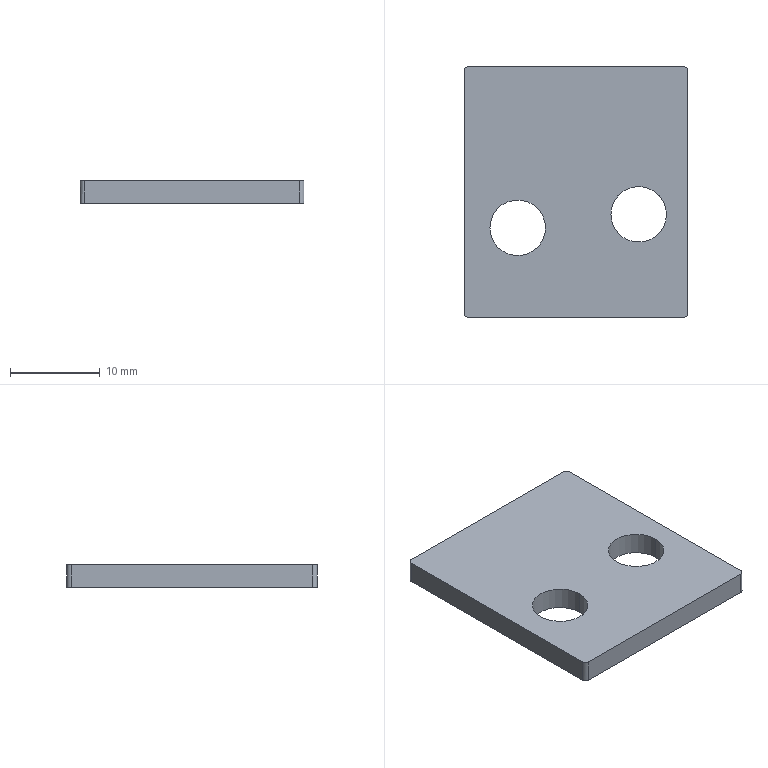Part | STEP file | PN_0024_Default<As Machined> | 1 solid | 14 faces | box 25 x 28 x 2.5 mm | volume 1599 mm3 | cylinder 8 | plane 6 | commonest cylinder face diameters 1 x4 6.2 x4
STEP:
#1=CARTESIAN_POINT('',(3.9,-2.5,2.5));
#2=VERTEX_POINT('',#1);
#3=CARTESIAN_POINT('',(10.1,-2.5,2.5));
#4=VERTEX_POINT('',#3);
#5=CARTESIAN_POINT('',(7.,-2.5,2.5));
#6=DIRECTION('',(0.,0.,-1.));
#7=AXIS2_PLACEMENT_3D('',#5,#6,$);
#8=CIRCLE('',#7,3.1);
#9=EDGE_CURVE('',#2,#4,#8,.F.);
#10=ORIENTED_EDGE('',*,*,#9,.T.);
#11=CARTESIAN_POINT('',(10.1,-2.5,0.));
#12=VERTEX_POINT('',#11);
#13=CARTESIAN_POINT('',(10.1,-2.5,2.5));
#14=DIRECTION('',(0.,0.,-1.));
#15=VECTOR('',#14,1.);
#16=LINE('',#13,#15);
#17=EDGE_CURVE('',#4,#12,#16,.T.);
#18=ORIENTED_EDGE('',*,*,#17,.T.);
#19=CARTESIAN_POINT('',(3.9,-2.5,0.));
#20=VERTEX_POINT('',#19);
#21=CARTESIAN_POINT('',(7.,-2.5,0.));
#22=DIRECTION('',(0.,0.,-1.));
#23=AXIS2_PLACEMENT_3D('',#21,#22,$);
#24=CIRCLE('',#23,3.1);
#25=EDGE_CURVE('',#20,#12,#24,.F.);
#26=ORIENTED_EDGE('',*,*,#25,.F.);
#27=CARTESIAN_POINT('',(3.9,-2.5,2.5));
#28=DIRECTION('',(0.,0.,-1.));
#29=VECTOR('',#28,1.);
#30=LINE('',#27,#29);
#31=EDGE_CURVE('',#2,#20,#30,.T.);
#32=ORIENTED_EDGE('',*,*,#31,.F.);
#33=EDGE_LOOP('',(#10,#18,#26,#32));
#34=FACE_OUTER_BOUND('',#33,.T.);
#35=CARTESIAN_POINT('',(7.,-2.5,2.5));
#36=DIRECTION('',(0.,0.,-1.));
#37=DIRECTION('',(1.,0.,0.));
#38=AXIS2_PLACEMENT_3D('',#35,#36,#37);
#39=CYLINDRICAL_SURFACE('',#38,3.1);
#40=ADVANCED_FACE('',(#34),#39,.F.);
#41=CARTESIAN_POINT('',(12.,14.,2.5));
#42=VERTEX_POINT('',#41);
#43=CARTESIAN_POINT('',(-12.,14.,2.5));
#44=VERTEX_POINT('',#43);
#45=CARTESIAN_POINT('',(0.,14.,2.5));
#46=DIRECTION('',(-1.,0.,0.));
#47=VECTOR('',#46,1.);
#48=LINE('',#45,#47);
#49=EDGE_CURVE('',#42,#44,#48,.T.);
#50=ORIENTED_EDGE('',*,*,#49,.T.);
#51=CARTESIAN_POINT('',(-12.5,13.5,2.5));
#52=VERTEX_POINT('',#51);
#53=CARTESIAN_POINT('',(-12.,13.5,2.5));
#54=DIRECTION('',(0.,0.,1.));
#55=AXIS2_PLACEMENT_3D('',#53,#54,$);
#56=CIRCLE('',#55,0.5);
#57=EDGE_CURVE('',#44,#52,#56,.T.);
#58=ORIENTED_EDGE('',*,*,#57,.T.);
#59=CARTESIAN_POINT('',(-12.5,-13.5,2.5));
#60=VERTEX_POINT('',#59);
#61=CARTESIAN_POINT('',(-12.5,0.,2.5));
#62=DIRECTION('',(0.,-1.,0.));
#63=VECTOR('',#62,1.);
#64=LINE('',#61,#63);
#65=EDGE_CURVE('',#52,#60,#64,.T.);
#66=ORIENTED_EDGE('',*,*,#65,.T.);
#67=CARTESIAN_POINT('',(-12.,-14.,2.5));
#68=VERTEX_POINT('',#67);
#69=CARTESIAN_POINT('',(-12.,-13.5,2.5));
#70=DIRECTION('',(0.,0.,1.));
#71=AXIS2_PLACEMENT_3D('',#69,#70,$);
#72=CIRCLE('',#71,0.5);
#73=EDGE_CURVE('',#60,#68,#72,.T.);
#74=ORIENTED_EDGE('',*,*,#73,.T.);
#75=CARTESIAN_POINT('',(12.,-14.,2.5));
#76=VERTEX_POINT('',#75);
#77=CARTESIAN_POINT('',(0.,-14.,2.5));
#78=DIRECTION('',(1.,0.,0.));
#79=VECTOR('',#78,1.);
#80=LINE('',#77,#79);
#81=EDGE_CURVE('',#68,#76,#80,.T.);
#82=ORIENTED_EDGE('',*,*,#81,.T.);
#83=CARTESIAN_POINT('',(12.5,-13.5,2.5));
#84=VERTEX_POINT('',#83);
#85=CARTESIAN_POINT('',(12.,-13.5,2.5));
#86=DIRECTION('',(0.,0.,1.));
#87=AXIS2_PLACEMENT_3D('',#85,#86,$);
#88=CIRCLE('',#87,0.5);
#89=EDGE_CURVE('',#76,#84,#88,.T.);
#90=ORIENTED_EDGE('',*,*,#89,.T.);
#91=CARTESIAN_POINT('',(12.5,13.5,2.5));
#92=VERTEX_POINT('',#91);
#93=CARTESIAN_POINT('',(12.5,0.,2.5));
#94=DIRECTION('',(0.,1.,0.));
#95=VECTOR('',#94,1.);
#96=LINE('',#93,#95);
#97=EDGE_CURVE('',#84,#92,#96,.T.);
#98=ORIENTED_EDGE('',*,*,#97,.T.);
#99=CARTESIAN_POINT('',(12.,13.5,2.5));
#100=DIRECTION('',(0.,0.,1.));
#101=AXIS2_PLACEMENT_3D('',#99,#100,$);
#102=CIRCLE('',#101,0.5);
#103=EDGE_CURVE('',#92,#42,#102,.T.);
#104=ORIENTED_EDGE('',*,*,#103,.T.);
#105=EDGE_LOOP('',(#50,#58,#66,#74,#82,#90,#98,#104));
#106=FACE_OUTER_BOUND('',#105,.T.);
#107=CARTESIAN_POINT('',(-9.6,-4.,2.5));
#108=VERTEX_POINT('',#107);
#109=CARTESIAN_POINT('',(-3.4,-4.,2.5));
#110=VERTEX_POINT('',#109);
#111=CARTESIAN_POINT('',(-6.5,-4.,2.5));
#112=DIRECTION('',(0.,0.,1.));
#113=AXIS2_PLACEMENT_3D('',#111,#112,$);
#114=CIRCLE('',#113,3.1);
#115=EDGE_CURVE('',#108,#110,#114,.T.);
#116=ORIENTED_EDGE('',*,*,#115,.F.);
#117=CARTESIAN_POINT('',(-6.5,-4.,2.5));
#118=DIRECTION('',(0.,0.,1.));
#119=AXIS2_PLACEMENT_3D('',#117,#118,$);
#120=CIRCLE('',#119,3.1);
#121=EDGE_CURVE('',#110,#108,#120,.T.);
#122=ORIENTED_EDGE('',*,*,#121,.F.);
#123=EDGE_LOOP('',(#116,#122));
#124=FACE_BOUND('',#123,.T.);
#125=ORIENTED_EDGE('',*,*,#9,.F.);
#126=CARTESIAN_POINT('',(7.,-2.5,2.5));
#127=DIRECTION('',(0.,0.,1.));
#128=AXIS2_PLACEMENT_3D('',#126,#127,$);
#129=CIRCLE('',#128,3.1);
#130=EDGE_CURVE('',#4,#2,#129,.T.);
#131=ORIENTED_EDGE('',*,*,#130,.F.);
#132=EDGE_LOOP('',(#125,#131));
#133=FACE_BOUND('',#132,.T.);
#134=CARTESIAN_POINT('',(0.,0.,2.5));
#135=DIRECTION('',(0.,0.,1.));
#136=DIRECTION('',(1.,0.,0.));
#137=AXIS2_PLACEMENT_3D('',#134,#135,#136);
#138=PLANE('',#137);
#139=ADVANCED_FACE('',(#106,#124,#133),#138,.T.);
#140=ORIENTED_EDGE('',*,*,#17,.F.);
#141=ORIENTED_EDGE('',*,*,#130,.T.);
#142=ORIENTED_EDGE('',*,*,#31,.T.);
#143=CARTESIAN_POINT('',(7.,-2.5,0.));
#144=DIRECTION('',(0.,0.,-1.));
#145=AXIS2_PLACEMENT_3D('',#143,#144,$);
#146=CIRCLE('',#145,3.1);
#147=EDGE_CURVE('',#12,#20,#146,.F.);
#148=ORIENTED_EDGE('',*,*,#147,.F.);
#149=EDGE_LOOP('',(#140,#141,#142,#148));
#150=FACE_OUTER_BOUND('',#149,.T.);
#151=CARTESIAN_POINT('',(7.,-2.5,2.5));
#152=DIRECTION('',(0.,0.,-1.));
#153=DIRECTION('',(-1.,0.,0.));
#154=AXIS2_PLACEMENT_3D('',#151,#152,#153);
#155=CYLINDRICAL_SURFACE('',#154,3.1);
#156=ADVANCED_FACE('',(#150),#155,.F.);
#157=CARTESIAN_POINT('',(-12.5,13.5,0.));
#158=VERTEX_POINT('',#157);
#159=CARTESIAN_POINT('',(-12.5,-13.5,0.));
#160=VERTEX_POINT('',#159);
#161=CARTESIAN_POINT('',(-12.5,0.,0.));
#162=DIRECTION('',(0.,-1.,0.));
#163=VECTOR('',#162,1.);
#164=LINE('',#161,#163);
#165=EDGE_CURVE('',#158,#160,#164,.T.);
#166=ORIENTED_EDGE('',*,*,#165,.F.);
#167=CARTESIAN_POINT('',(-12.,14.,0.));
#168=VERTEX_POINT('',#167);
#169=CARTESIAN_POINT('',(-12.5,13.5,0.));
#170=CARTESIAN_POINT('',(-12.5,13.563,0.));
#171=CARTESIAN_POINT('',(-12.49,13.626,0.));
#172=CARTESIAN_POINT('',(-12.47,13.686,0.));
#173=CARTESIAN_POINT('',(-12.412,13.8,0.));
#174=CARTESIAN_POINT('',(-12.323,13.89,0.));
#175=CARTESIAN_POINT('',(-12.271,13.927,0.));
#176=CARTESIAN_POINT('',(-12.186,13.97,0.));
#177=CARTESIAN_POINT('',(-12.094,13.993,0.));
#178=CARTESIAN_POINT('',(-12.063,13.998,0.));
#179=CARTESIAN_POINT('',(-12.031,14.,0.));
#180=CARTESIAN_POINT('',(-12.,14.,0.));
#181=B_SPLINE_CURVE_WITH_KNOTS('',5,(#169,#170,#171,#172,#173,#174,#175,#176,#177,#178,#179,#180),.UNSPECIFIED.,.F.,.U.,(6,3,3,6),(0.,0.4443,0.8886,1.11),.UNSPECIFIED.);
#182=EDGE_CURVE('',#158,#168,#181,.T.);
#183=ORIENTED_EDGE('',*,*,#182,.T.);
#184=CARTESIAN_POINT('',(12.,14.,0.));
#185=VERTEX_POINT('',#184);
#186=CARTESIAN_POINT('',(0.,14.,0.));
#187=DIRECTION('',(-1.,0.,0.));
#188=VECTOR('',#187,1.);
#189=LINE('',#186,#188);
#190=EDGE_CURVE('',#185,#168,#189,.T.);
#191=ORIENTED_EDGE('',*,*,#190,.F.);
#192=CARTESIAN_POINT('',(12.5,13.5,0.));
#193=VERTEX_POINT('',#192);
#194=CARTESIAN_POINT('',(12.,14.,0.));
#195=CARTESIAN_POINT('',(12.063,14.,0.));
#196=CARTESIAN_POINT('',(12.126,13.99,0.));
#197=CARTESIAN_POINT('',(12.186,13.97,0.));
#198=CARTESIAN_POINT('',(12.3,13.912,0.));
#199=CARTESIAN_POINT('',(12.39,13.823,0.));
#200=CARTESIAN_POINT('',(12.427,13.771,0.));
#201=CARTESIAN_POINT('',(12.47,13.686,0.));
#202=CARTESIAN_POINT('',(12.493,13.594,0.));
#203=CARTESIAN_POINT('',(12.498,13.563,0.));
#204=CARTESIAN_POINT('',(12.5,13.531,0.));
#205=CARTESIAN_POINT('',(12.5,13.5,0.));
#206=B_SPLINE_CURVE_WITH_KNOTS('',5,(#194,#195,#196,#197,#198,#199,#200,#201,#202,#203,#204,#205),.UNSPECIFIED.,.F.,.U.,(6,3,3,6),(0.,0.4443,0.8886,1.11),.UNSPECIFIED.);
#207=EDGE_CURVE('',#185,#193,#206,.T.);
#208=ORIENTED_EDGE('',*,*,#207,.T.);
#209=CARTESIAN_POINT('',(12.5,-13.5,0.));
#210=VERTEX_POINT('',#209);
#211=CARTESIAN_POINT('',(12.5,0.,0.));
#212=DIRECTION('',(0.,1.,0.));
#213=VECTOR('',#212,1.);
#214=LINE('',#211,#213);
#215=EDGE_CURVE('',#210,#193,#214,.T.);
#216=ORIENTED_EDGE('',*,*,#215,.F.);
#217=CARTESIAN_POINT('',(12.,-14.,0.));
#218=VERTEX_POINT('',#217);
#219=CARTESIAN_POINT('',(12.5,-13.5,0.));
#220=CARTESIAN_POINT('',(12.5,-13.563,0.));
#221=CARTESIAN_POINT('',(12.49,-13.626,0.));
#222=CARTESIAN_POINT('',(12.47,-13.686,0.));
#223=CARTESIAN_POINT('',(12.412,-13.8,0.));
#224=CARTESIAN_POINT('',(12.323,-13.89,0.));
#225=CARTESIAN_POINT('',(12.271,-13.927,0.));
#226=CARTESIAN_POINT('',(12.186,-13.97,0.));
#227=CARTESIAN_POINT('',(12.094,-13.993,0.));
#228=CARTESIAN_POINT('',(12.063,-13.998,0.));
#229=CARTESIAN_POINT('',(12.031,-14.,0.));
#230=CARTESIAN_POINT('',(12.,-14.,0.));
#231=B_SPLINE_CURVE_WITH_KNOTS('',5,(#219,#220,#221,#222,#223,#224,#225,#226,#227,#228,#229,#230),.UNSPECIFIED.,.F.,.U.,(6,3,3,6),(0.,0.4443,0.8886,1.11),.UNSPECIFIED.);
#232=EDGE_CURVE('',#210,#218,#231,.T.);
#233=ORIENTED_EDGE('',*,*,#232,.T.);
#234=CARTESIAN_POINT('',(-12.,-14.,0.));
#235=VERTEX_POINT('',#234);
#236=CARTESIAN_POINT('',(0.,-14.,0.));
#237=DIRECTION('',(1.,0.,0.));
#238=VECTOR('',#237,1.);
#239=LINE('',#236,#238);
#240=EDGE_CURVE('',#235,#218,#239,.T.);
#241=ORIENTED_EDGE('',*,*,#240,.F.);
#242=CARTESIAN_POINT('',(-12.,-14.,0.));
#243=CARTESIAN_POINT('',(-12.063,-14.,0.));
#244=CARTESIAN_POINT('',(-12.126,-13.99,0.));
#245=CARTESIAN_POINT('',(-12.186,-13.97,0.));
#246=CARTESIAN_POINT('',(-12.3,-13.912,0.));
#247=CARTESIAN_POINT('',(-12.39,-13.823,0.));
#248=CARTESIAN_POINT('',(-12.427,-13.771,0.));
#249=CARTESIAN_POINT('',(-12.47,-13.686,0.));
#250=CARTESIAN_POINT('',(-12.493,-13.594,0.));
#251=CARTESIAN_POINT('',(-12.498,-13.563,0.));
#252=CARTESIAN_POINT('',(-12.5,-13.531,0.));
#253=CARTESIAN_POINT('',(-12.5,-13.5,0.));
#254=B_SPLINE_CURVE_WITH_KNOTS('',5,(#242,#243,#244,#245,#246,#247,#248,#249,#250,#251,#252,#253),.UNSPECIFIED.,.F.,.U.,(6,3,3,6),(0.,0.4443,0.8886,1.11),.UNSPECIFIED.);
#255=EDGE_CURVE('',#235,#160,#254,.T.);
#256=ORIENTED_EDGE('',*,*,#255,.T.);
#257=EDGE_LOOP('',(#166,#183,#191,#208,#216,#233,#241,#256));
#258=FACE_OUTER_BOUND('',#257,.T.);
#259=CARTESIAN_POINT('',(-9.6,-4.,0.));
#260=VERTEX_POINT('',#259);
#261=CARTESIAN_POINT('',(-3.4,-4.,0.));
#262=VERTEX_POINT('',#261);
#263=CARTESIAN_POINT('',(-6.5,-4.,0.));
#264=DIRECTION('',(0.,0.,1.));
#265=AXIS2_PLACEMENT_3D('',#263,#264,$);
#266=CIRCLE('',#265,3.1);
#267=EDGE_CURVE('',#260,#262,#266,.T.);
#268=ORIENTED_EDGE('',*,*,#267,.T.);
#269=CARTESIAN_POINT('',(-6.5,-4.,0.));
#270=DIRECTION('',(0.,0.,1.));
#271=AXIS2_PLACEMENT_3D('',#269,#270,$);
#272=CIRCLE('',#271,3.1);
#273=EDGE_CURVE('',#262,#260,#272,.T.);
#274=ORIENTED_EDGE('',*,*,#273,.T.);
#275=EDGE_LOOP('',(#268,#274));
#276=FACE_BOUND('',#275,.T.);
#277=ORIENTED_EDGE('',*,*,#25,.T.);
#278=ORIENTED_EDGE('',*,*,#147,.T.);
#279=EDGE_LOOP('',(#277,#278));
#280=FACE_BOUND('',#279,.T.);
#281=CARTESIAN_POINT('',(0.,0.,0.));
#282=DIRECTION('',(0.,0.,1.));
#283=DIRECTION('',(1.,0.,0.));
#284=AXIS2_PLACEMENT_3D('',#281,#282,#283);
#285=PLANE('',#284);
#286=ADVANCED_FACE('',(#258,#276,#280),#285,.F.);
#287=ORIENTED_EDGE('',*,*,#190,.T.);
#288=CARTESIAN_POINT('',(-12.,14.,1.25));
#289=DIRECTION('',(0.,0.,1.));
#290=VECTOR('',#289,1.);
#291=LINE('',#288,#290);
#292=EDGE_CURVE('',#168,#44,#291,.T.);
#293=ORIENTED_EDGE('',*,*,#292,.T.);
#294=ORIENTED_EDGE('',*,*,#49,.F.);
#295=CARTESIAN_POINT('',(12.,14.,1.25));
#296=DIRECTION('',(0.,0.,-1.));
#297=VECTOR('',#296,1.);
#298=LINE('',#295,#297);
#299=EDGE_CURVE('',#42,#185,#298,.T.);
#300=ORIENTED_EDGE('',*,*,#299,.T.);
#301=EDGE_LOOP('',(#287,#293,#294,#300));
#302=FACE_OUTER_BOUND('',#301,.T.);
#303=CARTESIAN_POINT('',(12.5,14.,2.5));
#304=DIRECTION('',(0.,-1.,0.));
#305=DIRECTION('',(1.,0.,0.));
#306=AXIS2_PLACEMENT_3D('',#303,#304,#305);
#307=PLANE('',#306);
#308=ADVANCED_FACE('',(#302),#307,.F.);
#309=ORIENTED_EDGE('',*,*,#57,.F.);
#310=ORIENTED_EDGE('',*,*,#292,.F.);
#311=ORIENTED_EDGE('',*,*,#182,.F.);
#312=CARTESIAN_POINT('',(-12.5,13.5,2.5));
#313=DIRECTION('',(0.,0.,-1.));
#314=VECTOR('',#313,1.);
#315=LINE('',#312,#314);
#316=EDGE_CURVE('',#52,#158,#315,.T.);
#317=ORIENTED_EDGE('',*,*,#316,.F.);
#318=EDGE_LOOP('',(#309,#310,#311,#317));
#319=FACE_OUTER_BOUND('',#318,.T.);
#320=CARTESIAN_POINT('',(-12.,13.5,2.5));
#321=DIRECTION('',(0.,0.,-1.));
#322=DIRECTION('',(-1.,0.,0.));
#323=AXIS2_PLACEMENT_3D('',#320,#321,#322);
#324=CYLINDRICAL_SURFACE('',#323,0.5);
#325=ADVANCED_FACE('',(#319),#324,.T.);
#326=ORIENTED_EDGE('',*,*,#65,.F.);
#327=ORIENTED_EDGE('',*,*,#316,.T.);
#328=ORIENTED_EDGE('',*,*,#165,.T.);
#329=CARTESIAN_POINT('',(-12.5,-13.5,1.25));
#330=DIRECTION('',(0.,0.,1.));
#331=VECTOR('',#330,1.);
#332=LINE('',#329,#331);
#333=EDGE_CURVE('',#160,#60,#332,.T.);
#334=ORIENTED_EDGE('',*,*,#333,.T.);
#335=EDGE_LOOP('',(#326,#327,#328,#334));
#336=FACE_OUTER_BOUND('',#335,.T.);
#337=CARTESIAN_POINT('',(-12.5,-14.,2.5));
#338=DIRECTION('',(1.,0.,0.));
#339=DIRECTION('',(0.,0.,-1.));
#340=AXIS2_PLACEMENT_3D('',#337,#338,#339);
#341=PLANE('',#340);
#342=ADVANCED_FACE('',(#336),#341,.F.);
#343=ORIENTED_EDGE('',*,*,#73,.F.);
#344=ORIENTED_EDGE('',*,*,#333,.F.);
#345=ORIENTED_EDGE('',*,*,#255,.F.);
#346=CARTESIAN_POINT('',(-12.,-14.,2.5));
#347=DIRECTION('',(0.,0.,-1.));
#348=VECTOR('',#347,1.);
#349=LINE('',#346,#348);
#350=EDGE_CURVE('',#68,#235,#349,.T.);
#351=ORIENTED_EDGE('',*,*,#350,.F.);
#352=EDGE_LOOP('',(#343,#344,#345,#351));
#353=FACE_OUTER_BOUND('',#352,.T.);
#354=CARTESIAN_POINT('',(-12.,-13.5,2.5));
#355=DIRECTION('',(0.,0.,-1.));
#356=DIRECTION('',(1.,0.,0.));
#357=AXIS2_PLACEMENT_3D('',#354,#355,#356);
#358=CYLINDRICAL_SURFACE('',#357,0.5);
#359=ADVANCED_FACE('',(#353),#358,.T.);
#360=ORIENTED_EDGE('',*,*,#240,.T.);
#361=CARTESIAN_POINT('',(12.,-14.,1.25));
#362=DIRECTION('',(0.,0.,1.));
#363=VECTOR('',#362,1.);
#364=LINE('',#361,#363);
#365=EDGE_CURVE('',#218,#76,#364,.T.);
#366=ORIENTED_EDGE('',*,*,#365,.T.);
#367=ORIENTED_EDGE('',*,*,#81,.F.);
#368=ORIENTED_EDGE('',*,*,#350,.T.);
#369=EDGE_LOOP('',(#360,#366,#367,#368));
#370=FACE_OUTER_BOUND('',#369,.T.);
#371=CARTESIAN_POINT('',(12.5,-14.,2.5));
#372=DIRECTION('',(0.,1.,0.));
#373=DIRECTION('',(-1.,0.,0.));
#374=AXIS2_PLACEMENT_3D('',#371,#372,#373);
#375=PLANE('',#374);
#376=ADVANCED_FACE('',(#370),#375,.F.);
#377=ORIENTED_EDGE('',*,*,#89,.F.);
#378=ORIENTED_EDGE('',*,*,#365,.F.);
#379=ORIENTED_EDGE('',*,*,#232,.F.);
#380=CARTESIAN_POINT('',(12.5,-13.5,2.5));
#381=DIRECTION('',(0.,0.,-1.));
#382=VECTOR('',#381,1.);
#383=LINE('',#380,#382);
#384=EDGE_CURVE('',#84,#210,#383,.T.);
#385=ORIENTED_EDGE('',*,*,#384,.F.);
#386=EDGE_LOOP('',(#377,#378,#379,#385));
#387=FACE_OUTER_BOUND('',#386,.T.);
#388=CARTESIAN_POINT('',(12.,-13.5,2.5));
#389=DIRECTION('',(0.,0.,-1.));
#390=DIRECTION('',(1.,0.,0.));
#391=AXIS2_PLACEMENT_3D('',#388,#389,#390);
#392=CYLINDRICAL_SURFACE('',#391,0.5);
#393=ADVANCED_FACE('',(#387),#392,.T.);
#394=ORIENTED_EDGE('',*,*,#97,.F.);
#395=ORIENTED_EDGE('',*,*,#384,.T.);
#396=ORIENTED_EDGE('',*,*,#215,.T.);
#397=CARTESIAN_POINT('',(12.5,13.5,1.25));
#398=DIRECTION('',(0.,0.,1.));
#399=VECTOR('',#398,1.);
#400=LINE('',#397,#399);
#401=EDGE_CURVE('',#193,#92,#400,.T.);
#402=ORIENTED_EDGE('',*,*,#401,.T.);
#403=EDGE_LOOP('',(#394,#395,#396,#402));
#404=FACE_OUTER_BOUND('',#403,.T.);
#405=CARTESIAN_POINT('',(12.5,-14.,2.5));
#406=DIRECTION('',(-1.,0.,0.));
#407=DIRECTION('',(0.,0.,1.));
#408=AXIS2_PLACEMENT_3D('',#405,#406,#407);
#409=PLANE('',#408);
#410=ADVANCED_FACE('',(#404),#409,.F.);
#411=ORIENTED_EDGE('',*,*,#103,.F.);
#412=ORIENTED_EDGE('',*,*,#401,.F.);
#413=ORIENTED_EDGE('',*,*,#207,.F.);
#414=ORIENTED_EDGE('',*,*,#299,.F.);
#415=EDGE_LOOP('',(#411,#412,#413,#414));
#416=FACE_OUTER_BOUND('',#415,.T.);
#417=CARTESIAN_POINT('',(12.,13.5,2.5));
#418=DIRECTION('',(0.,0.,-1.));
#419=DIRECTION('',(-1.,0.,0.));
#420=AXIS2_PLACEMENT_3D('',#417,#418,#419);
#421=CYLINDRICAL_SURFACE('',#420,0.5);
#422=ADVANCED_FACE('',(#416),#421,.T.);
#423=ORIENTED_EDGE('',*,*,#115,.T.);
#424=CARTESIAN_POINT('',(-3.4,-4.,2.5));
#425=DIRECTION('',(0.,0.,-1.));
#426=VECTOR('',#425,1.);
#427=LINE('',#424,#426);
#428=EDGE_CURVE('',#110,#262,#427,.T.);
#429=ORIENTED_EDGE('',*,*,#428,.T.);
#430=ORIENTED_EDGE('',*,*,#267,.F.);
#431=CARTESIAN_POINT('',(-9.6,-4.,2.5));
#432=DIRECTION('',(0.,0.,-1.));
#433=VECTOR('',#432,1.);
#434=LINE('',#431,#433);
#435=EDGE_CURVE('',#108,#260,#434,.T.);
#436=ORIENTED_EDGE('',*,*,#435,.F.);
#437=EDGE_LOOP('',(#423,#429,#430,#436));
#438=FACE_OUTER_BOUND('',#437,.T.);
#439=CARTESIAN_POINT('',(-6.5,-4.,2.5));
#440=DIRECTION('',(0.,0.,-1.));
#441=DIRECTION('',(1.,0.,0.));
#442=AXIS2_PLACEMENT_3D('',#439,#440,#441);
#443=CYLINDRICAL_SURFACE('',#442,3.1);
#444=ADVANCED_FACE('',(#438),#443,.F.);
#445=ORIENTED_EDGE('',*,*,#428,.F.);
#446=ORIENTED_EDGE('',*,*,#121,.T.);
#447=ORIENTED_EDGE('',*,*,#435,.T.);
#448=ORIENTED_EDGE('',*,*,#273,.F.);
#449=EDGE_LOOP('',(#445,#446,#447,#448));
#450=FACE_OUTER_BOUND('',#449,.T.);
#451=CARTESIAN_POINT('',(-6.5,-4.,2.5));
#452=DIRECTION('',(0.,0.,-1.));
#453=DIRECTION('',(-1.,0.,0.));
#454=AXIS2_PLACEMENT_3D('',#451,#452,#453);
#455=CYLINDRICAL_SURFACE('',#454,3.1);
#456=ADVANCED_FACE('',(#450),#455,.F.);
#457=CLOSED_SHELL('',(#40,#139,#156,#286,#308,#325,#342,#359,#376,#393,#410,#422,#444,#456));
#458=MANIFOLD_SOLID_BREP('',#457);
#459=(LENGTH_UNIT()NAMED_UNIT(*)SI_UNIT(.MILLI.,.METRE.));
#460=UNCERTAINTY_MEASURE_WITH_UNIT(LENGTH_MEASURE(0.005),#459,'','');
#461=(NAMED_UNIT(*)PLANE_ANGLE_UNIT()SI_UNIT($,.RADIAN.));
#462=(NAMED_UNIT(*)SI_UNIT($,.STERADIAN.)SOLID_ANGLE_UNIT());
#463=(GEOMETRIC_REPRESENTATION_CONTEXT(3)GLOBAL_UNCERTAINTY_ASSIGNED_CONTEXT((#460))GLOBAL_UNIT_ASSIGNED_CONTEXT((#459,#461,#462))REPRESENTATION_CONTEXT('',''));
#464=ADVANCED_BREP_SHAPE_REPRESENTATION('',(#458),#463);